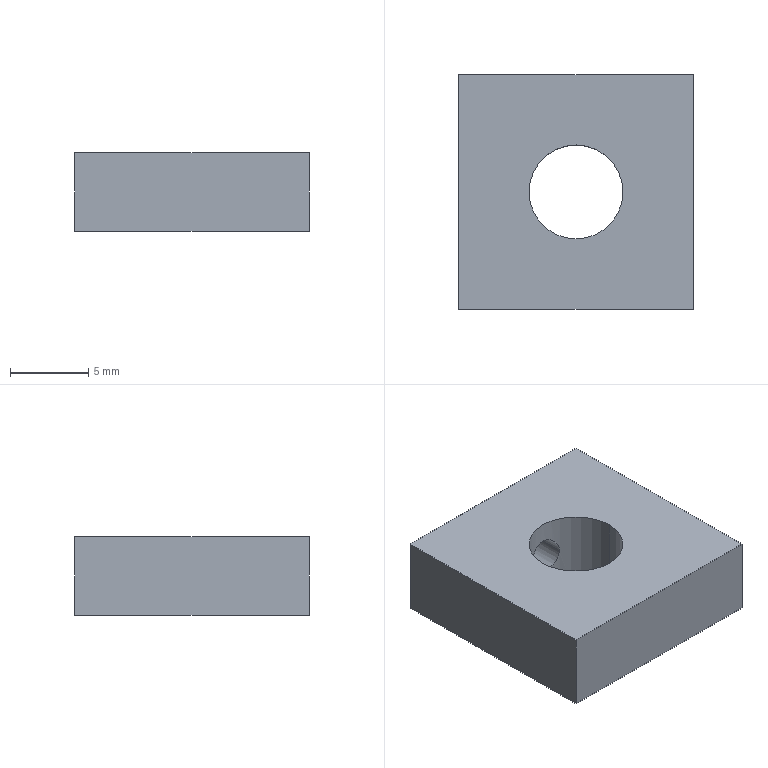Part | SolidWorks | features BaseBody 1 | 1 solid | 10 faces | box 15 x 15 x 5 mm | volume 961.952 mm3 | plane 6 | cylinder 4 | commonest cylinder face diameters 2.459 x2 6 x2
STEP:
#1=CARTESIAN_POINT('',(-105.792,-7.5,0.));
#2=VERTEX_POINT('',#1);
#3=CARTESIAN_POINT('',(-99.792,-7.5,0.));
#4=VERTEX_POINT('',#3);
#5=CARTESIAN_POINT('',(-102.792,-7.5,0.));
#6=DIRECTION('',(0.,0.,1.));
#7=DIRECTION('',(1.,0.,0.));
#8=AXIS2_PLACEMENT_3D('',#5,#6,#7);
#9=CIRCLE('',#8,3.);
#10=EDGE_CURVE('',#2,#4,#9,.T.);
#11=ORIENTED_EDGE('',*,*,#10,.F.);
#12=CARTESIAN_POINT('',(-105.792,-7.5,5.));
#13=VERTEX_POINT('',#12);
#14=CARTESIAN_POINT('',(-105.792,-7.5,-16.794));
#15=DIRECTION('',(0.,0.,1.));
#16=VECTOR('',#15,1000.);
#17=LINE('',#14,#16);
#18=EDGE_CURVE('',#2,#13,#17,.T.);
#19=ORIENTED_EDGE('',*,*,#18,.T.);
#20=CARTESIAN_POINT('',(-99.792,-7.5,5.));
#21=VERTEX_POINT('',#20);
#22=CARTESIAN_POINT('',(-102.792,-7.5,5.));
#23=DIRECTION('',(0.,0.,-1.));
#24=DIRECTION('',(1.,0.,0.));
#25=AXIS2_PLACEMENT_3D('',#22,#23,#24);
#26=CIRCLE('',#25,3.);
#27=EDGE_CURVE('',#21,#13,#26,.T.);
#28=ORIENTED_EDGE('',*,*,#27,.F.);
#29=CARTESIAN_POINT('',(-99.792,-7.5,-16.794));
#30=DIRECTION('',(0.,0.,1.));
#31=VECTOR('',#30,1000.);
#32=LINE('',#29,#31);
#33=EDGE_CURVE('',#4,#21,#32,.T.);
#34=ORIENTED_EDGE('',*,*,#33,.F.);
#35=EDGE_LOOP('',(#11,#19,#28,#34));
#36=FACE_OUTER_BOUND('',#35,.T.);
#37=CARTESIAN_POINT('',(-102.792,-7.5,-16.794));
#38=DIRECTION('',(0.,0.,1.));
#39=DIRECTION('',(1.,0.,0.));
#40=AXIS2_PLACEMENT_3D('',#37,#38,#39);
#41=CYLINDRICAL_SURFACE('',#40,3.);
#42=ADVANCED_FACE('',(#36),#41,.F.);
#43=CARTESIAN_POINT('',(-104.021,-4.764,2.5));
#44=VERTEX_POINT('',#43);
#45=CARTESIAN_POINT('',(-101.562,-4.764,2.5));
#46=VERTEX_POINT('',#45);
#47=CARTESIAN_POINT('',(-104.021,-4.764,2.5));
#48=CARTESIAN_POINT('',(-104.021,-4.764,2.336));
#49=CARTESIAN_POINT('',(-103.988,-4.748,2.174));
#50=CARTESIAN_POINT('',(-103.864,-4.697,1.878));
#51=CARTESIAN_POINT('',(-103.773,-4.663,1.743));
#52=CARTESIAN_POINT('',(-103.549,-4.595,1.518));
#53=CARTESIAN_POINT('',(-103.413,-4.561,1.427));
#54=CARTESIAN_POINT('',(-103.118,-4.514,1.304));
#55=CARTESIAN_POINT('',(-102.955,-4.5,1.271));
#56=CARTESIAN_POINT('',(-102.711,-4.5,1.27));
#57=CARTESIAN_POINT('',(-102.629,-4.503,1.279));
#58=CARTESIAN_POINT('',(-102.47,-4.516,1.311));
#59=CARTESIAN_POINT('',(-102.393,-4.526,1.334));
#60=CARTESIAN_POINT('',(-102.168,-4.562,1.428));
#61=CARTESIAN_POINT('',(-102.034,-4.595,1.519));
#62=CARTESIAN_POINT('',(-101.809,-4.663,1.744));
#63=CARTESIAN_POINT('',(-101.718,-4.698,1.879));
#64=CARTESIAN_POINT('',(-101.595,-4.748,2.175));
#65=CARTESIAN_POINT('',(-101.562,-4.764,2.338));
#66=CARTESIAN_POINT('',(-101.562,-4.764,2.5));
#67=B_SPLINE_CURVE_WITH_KNOTS('',3,(#47,#48,#49,#50,#51,#52,#53,#54,#55,#56,#57,#58,#59,#60,#61,#62,#63,#64,#65,#66),.UNSPECIFIED.,.F.,.F.,(4,2,2,2,2,2,2,2,2,4),(0.,0.0004859,0.0009718,0.001458,0.001944,0.002186,0.002429,0.002915,0.003401,0.003887),.UNSPECIFIED.);
#68=EDGE_CURVE('',#44,#46,#67,.T.);
#69=ORIENTED_EDGE('',*,*,#68,.T.);
#70=CARTESIAN_POINT('',(-101.562,0.,2.5));
#71=VERTEX_POINT('',#70);
#72=CARTESIAN_POINT('',(-101.562,-4.,2.5));
#73=DIRECTION('',(0.,1.,0.));
#74=VECTOR('',#73,1000.);
#75=LINE('',#72,#74);
#76=EDGE_CURVE('',#46,#71,#75,.T.);
#77=ORIENTED_EDGE('',*,*,#76,.T.);
#78=CARTESIAN_POINT('',(-104.021,0.,2.5));
#79=VERTEX_POINT('',#78);
#80=CARTESIAN_POINT('',(-102.792,0.,2.5));
#81=DIRECTION('',(0.,-1.,0.));
#82=DIRECTION('',(-1.,0.,0.));
#83=AXIS2_PLACEMENT_3D('',#80,#81,#82);
#84=CIRCLE('',#83,1.229);
#85=EDGE_CURVE('',#79,#71,#84,.T.);
#86=ORIENTED_EDGE('',*,*,#85,.F.);
#87=CARTESIAN_POINT('',(-104.021,-4.,2.5));
#88=DIRECTION('',(0.,1.,0.));
#89=VECTOR('',#88,1000.);
#90=LINE('',#87,#89);
#91=EDGE_CURVE('',#44,#79,#90,.T.);
#92=ORIENTED_EDGE('',*,*,#91,.F.);
#93=EDGE_LOOP('',(#69,#77,#86,#92));
#94=FACE_OUTER_BOUND('',#93,.T.);
#95=CARTESIAN_POINT('',(-102.792,-4.,2.5));
#96=DIRECTION('',(0.,1.,0.));
#97=DIRECTION('',(-1.,0.,0.));
#98=AXIS2_PLACEMENT_3D('',#95,#96,#97);
#99=CYLINDRICAL_SURFACE('',#98,1.229);
#100=ADVANCED_FACE('',(#94),#99,.F.);
#101=ORIENTED_EDGE('',*,*,#27,.T.);
#102=CARTESIAN_POINT('',(-102.792,-7.5,5.));
#103=DIRECTION('',(0.,0.,-1.));
#104=DIRECTION('',(1.,0.,0.));
#105=AXIS2_PLACEMENT_3D('',#102,#103,#104);
#106=CIRCLE('',#105,3.);
#107=EDGE_CURVE('',#13,#21,#106,.T.);
#108=ORIENTED_EDGE('',*,*,#107,.T.);
#109=EDGE_LOOP('',(#101,#108));
#110=FACE_BOUND('',#109,.T.);
#111=CARTESIAN_POINT('',(-95.292,-15.,5.));
#112=VERTEX_POINT('',#111);
#113=CARTESIAN_POINT('',(-95.292,0.,5.));
#114=VERTEX_POINT('',#113);
#115=CARTESIAN_POINT('',(-95.292,-7.5,5.));
#116=DIRECTION('',(0.,1.,0.));
#117=VECTOR('',#116,1000.);
#118=LINE('',#115,#117);
#119=EDGE_CURVE('',#112,#114,#118,.T.);
#120=ORIENTED_EDGE('',*,*,#119,.T.);
#121=CARTESIAN_POINT('',(-110.292,0.,5.));
#122=VERTEX_POINT('',#121);
#123=CARTESIAN_POINT('',(-102.792,0.,5.));
#124=DIRECTION('',(-1.,0.,0.));
#125=VECTOR('',#124,1000.);
#126=LINE('',#123,#125);
#127=EDGE_CURVE('',#114,#122,#126,.T.);
#128=ORIENTED_EDGE('',*,*,#127,.T.);
#129=CARTESIAN_POINT('',(-110.292,-15.,5.));
#130=VERTEX_POINT('',#129);
#131=CARTESIAN_POINT('',(-110.292,-7.5,5.));
#132=DIRECTION('',(0.,-1.,0.));
#133=VECTOR('',#132,1000.);
#134=LINE('',#131,#133);
#135=EDGE_CURVE('',#122,#130,#134,.T.);
#136=ORIENTED_EDGE('',*,*,#135,.T.);
#137=CARTESIAN_POINT('',(-102.792,-15.,5.));
#138=DIRECTION('',(1.,0.,0.));
#139=VECTOR('',#138,1000.);
#140=LINE('',#137,#139);
#141=EDGE_CURVE('',#130,#112,#140,.T.);
#142=ORIENTED_EDGE('',*,*,#141,.T.);
#143=EDGE_LOOP('',(#120,#128,#136,#142));
#144=FACE_OUTER_BOUND('',#143,.T.);
#145=CARTESIAN_POINT('',(-102.792,-7.5,5.));
#146=DIRECTION('',(0.,0.,1.));
#147=DIRECTION('',(1.,0.,0.));
#148=AXIS2_PLACEMENT_3D('',#145,#146,#147);
#149=PLANE('',#148);
#150=ADVANCED_FACE('',(#110,#144),#149,.T.);
#151=ORIENTED_EDGE('',*,*,#18,.F.);
#152=CARTESIAN_POINT('',(-102.792,-7.5,0.));
#153=DIRECTION('',(0.,0.,1.));
#154=DIRECTION('',(1.,0.,0.));
#155=AXIS2_PLACEMENT_3D('',#152,#153,#154);
#156=CIRCLE('',#155,3.);
#157=EDGE_CURVE('',#4,#2,#156,.T.);
#158=ORIENTED_EDGE('',*,*,#157,.F.);
#159=ORIENTED_EDGE('',*,*,#33,.T.);
#160=ORIENTED_EDGE('',*,*,#107,.F.);
#161=EDGE_LOOP('',(#151,#158,#159,#160));
#162=FACE_OUTER_BOUND('',#161,.T.);
#163=ORIENTED_EDGE('',*,*,#68,.F.);
#164=CARTESIAN_POINT('',(-101.562,-4.764,2.5));
#165=CARTESIAN_POINT('',(-101.562,-4.764,2.662));
#166=CARTESIAN_POINT('',(-101.595,-4.748,2.825));
#167=CARTESIAN_POINT('',(-101.719,-4.698,3.122));
#168=CARTESIAN_POINT('',(-101.809,-4.663,3.256));
#169=CARTESIAN_POINT('',(-101.979,-4.612,3.426));
#170=CARTESIAN_POINT('',(-102.041,-4.595,3.477));
#171=CARTESIAN_POINT('',(-102.173,-4.564,3.565));
#172=CARTESIAN_POINT('',(-102.244,-4.549,3.604));
#173=CARTESIAN_POINT('',(-102.393,-4.526,3.666));
#174=CARTESIAN_POINT('',(-102.47,-4.516,3.689));
#175=CARTESIAN_POINT('',(-102.628,-4.503,3.721));
#176=CARTESIAN_POINT('',(-102.711,-4.5,3.729));
#177=CARTESIAN_POINT('',(-102.954,-4.5,3.73));
#178=CARTESIAN_POINT('',(-103.117,-4.514,3.697));
#179=CARTESIAN_POINT('',(-103.414,-4.561,3.573));
#180=CARTESIAN_POINT('',(-103.549,-4.595,3.482));
#181=CARTESIAN_POINT('',(-103.774,-4.663,3.256));
#182=CARTESIAN_POINT('',(-103.864,-4.697,3.123));
#183=CARTESIAN_POINT('',(-103.989,-4.748,2.824));
#184=CARTESIAN_POINT('',(-104.021,-4.764,2.664));
#185=CARTESIAN_POINT('',(-104.021,-4.764,2.5));
#186=B_SPLINE_CURVE_WITH_KNOTS('',3,(#164,#165,#166,#167,#168,#169,#170,#171,#172,#173,#174,#175,#176,#177,#178,#179,#180,#181,#182,#183,#184,#185),.UNSPECIFIED.,.F.,.F.,(4,2,2,2,2,2,2,2,2,2,4),(0.003887,0.004373,0.004858,0.005101,0.005344,0.005586,0.005829,0.006315,0.0068,0.007286,0.007771),.UNSPECIFIED.);
#187=EDGE_CURVE('',#46,#44,#186,.T.);
#188=ORIENTED_EDGE('',*,*,#187,.F.);
#189=EDGE_LOOP('',(#163,#188));
#190=FACE_BOUND('',#189,.T.);
#191=CARTESIAN_POINT('',(-102.792,-7.5,-16.794));
#192=DIRECTION('',(0.,0.,1.));
#193=DIRECTION('',(1.,0.,0.));
#194=AXIS2_PLACEMENT_3D('',#191,#192,#193);
#195=CYLINDRICAL_SURFACE('',#194,3.);
#196=ADVANCED_FACE('',(#162,#190),#195,.F.);
#197=ORIENTED_EDGE('',*,*,#85,.T.);
#198=CARTESIAN_POINT('',(-102.792,0.,2.5));
#199=DIRECTION('',(0.,-1.,0.));
#200=DIRECTION('',(-1.,0.,0.));
#201=AXIS2_PLACEMENT_3D('',#198,#199,#200);
#202=CIRCLE('',#201,1.229);
#203=EDGE_CURVE('',#71,#79,#202,.T.);
#204=ORIENTED_EDGE('',*,*,#203,.T.);
#205=EDGE_LOOP('',(#197,#204));
#206=FACE_BOUND('',#205,.T.);
#207=CARTESIAN_POINT('',(-95.292,0.,0.));
#208=VERTEX_POINT('',#207);
#209=CARTESIAN_POINT('',(-110.292,0.,0.));
#210=VERTEX_POINT('',#209);
#211=CARTESIAN_POINT('',(-110.292,0.,0.));
#212=DIRECTION('',(-1.,0.,0.));
#213=VECTOR('',#212,1000.);
#214=LINE('',#211,#213);
#215=EDGE_CURVE('',#208,#210,#214,.T.);
#216=ORIENTED_EDGE('',*,*,#215,.T.);
#217=CARTESIAN_POINT('',(-110.292,0.,0.));
#218=DIRECTION('',(0.,0.,1.));
#219=VECTOR('',#218,1000.);
#220=LINE('',#217,#219);
#221=EDGE_CURVE('',#210,#122,#220,.T.);
#222=ORIENTED_EDGE('',*,*,#221,.T.);
#223=ORIENTED_EDGE('',*,*,#127,.F.);
#224=CARTESIAN_POINT('',(-95.292,0.,0.));
#225=DIRECTION('',(0.,0.,-1.));
#226=VECTOR('',#225,1000.);
#227=LINE('',#224,#226);
#228=EDGE_CURVE('',#114,#208,#227,.T.);
#229=ORIENTED_EDGE('',*,*,#228,.T.);
#230=EDGE_LOOP('',(#216,#222,#223,#229));
#231=FACE_OUTER_BOUND('',#230,.T.);
#232=CARTESIAN_POINT('',(-110.292,0.,0.));
#233=DIRECTION('',(0.,1.,0.));
#234=DIRECTION('',(0.,0.,1.));
#235=AXIS2_PLACEMENT_3D('',#232,#233,#234);
#236=PLANE('',#235);
#237=ADVANCED_FACE('',(#206,#231),#236,.T.);
#238=CARTESIAN_POINT('',(-95.292,-15.,0.));
#239=VERTEX_POINT('',#238);
#240=CARTESIAN_POINT('',(-95.292,0.,0.));
#241=DIRECTION('',(0.,1.,0.));
#242=VECTOR('',#241,1000.);
#243=LINE('',#240,#242);
#244=EDGE_CURVE('',#239,#208,#243,.T.);
#245=ORIENTED_EDGE('',*,*,#244,.T.);
#246=ORIENTED_EDGE('',*,*,#228,.F.);
#247=ORIENTED_EDGE('',*,*,#119,.F.);
#248=CARTESIAN_POINT('',(-95.292,-15.,0.));
#249=DIRECTION('',(0.,0.,-1.));
#250=VECTOR('',#249,1000.);
#251=LINE('',#248,#250);
#252=EDGE_CURVE('',#112,#239,#251,.T.);
#253=ORIENTED_EDGE('',*,*,#252,.T.);
#254=EDGE_LOOP('',(#245,#246,#247,#253));
#255=FACE_OUTER_BOUND('',#254,.T.);
#256=CARTESIAN_POINT('',(-95.292,0.,0.));
#257=DIRECTION('',(1.,0.,0.));
#258=DIRECTION('',(0.,0.,-1.));
#259=AXIS2_PLACEMENT_3D('',#256,#257,#258);
#260=PLANE('',#259);
#261=ADVANCED_FACE('',(#255),#260,.T.);
#262=CARTESIAN_POINT('',(-110.292,-15.,0.));
#263=VERTEX_POINT('',#262);
#264=CARTESIAN_POINT('',(-95.292,-15.,0.));
#265=DIRECTION('',(1.,0.,0.));
#266=VECTOR('',#265,1000.);
#267=LINE('',#264,#266);
#268=EDGE_CURVE('',#263,#239,#267,.T.);
#269=ORIENTED_EDGE('',*,*,#268,.T.);
#270=ORIENTED_EDGE('',*,*,#252,.F.);
#271=ORIENTED_EDGE('',*,*,#141,.F.);
#272=CARTESIAN_POINT('',(-110.292,-15.,0.));
#273=DIRECTION('',(0.,0.,-1.));
#274=VECTOR('',#273,1000.);
#275=LINE('',#272,#274);
#276=EDGE_CURVE('',#130,#263,#275,.T.);
#277=ORIENTED_EDGE('',*,*,#276,.T.);
#278=EDGE_LOOP('',(#269,#270,#271,#277));
#279=FACE_OUTER_BOUND('',#278,.T.);
#280=CARTESIAN_POINT('',(-95.292,-15.,0.));
#281=DIRECTION('',(0.,-1.,0.));
#282=DIRECTION('',(0.,0.,-1.));
#283=AXIS2_PLACEMENT_3D('',#280,#281,#282);
#284=PLANE('',#283);
#285=ADVANCED_FACE('',(#279),#284,.T.);
#286=CARTESIAN_POINT('',(-110.292,-15.,0.));
#287=DIRECTION('',(0.,-1.,0.));
#288=VECTOR('',#287,1000.);
#289=LINE('',#286,#288);
#290=EDGE_CURVE('',#210,#263,#289,.T.);
#291=ORIENTED_EDGE('',*,*,#290,.T.);
#292=ORIENTED_EDGE('',*,*,#276,.F.);
#293=ORIENTED_EDGE('',*,*,#135,.F.);
#294=ORIENTED_EDGE('',*,*,#221,.F.);
#295=EDGE_LOOP('',(#291,#292,#293,#294));
#296=FACE_OUTER_BOUND('',#295,.T.);
#297=CARTESIAN_POINT('',(-110.292,-15.,0.));
#298=DIRECTION('',(-1.,0.,0.));
#299=DIRECTION('',(0.,0.,1.));
#300=AXIS2_PLACEMENT_3D('',#297,#298,#299);
#301=PLANE('',#300);
#302=ADVANCED_FACE('',(#296),#301,.T.);
#303=ORIENTED_EDGE('',*,*,#76,.F.);
#304=ORIENTED_EDGE('',*,*,#187,.T.);
#305=ORIENTED_EDGE('',*,*,#91,.T.);
#306=ORIENTED_EDGE('',*,*,#203,.F.);
#307=EDGE_LOOP('',(#303,#304,#305,#306));
#308=FACE_OUTER_BOUND('',#307,.T.);
#309=CARTESIAN_POINT('',(-102.792,-4.,2.5));
#310=DIRECTION('',(0.,1.,0.));
#311=DIRECTION('',(-1.,0.,0.));
#312=AXIS2_PLACEMENT_3D('',#309,#310,#311);
#313=CYLINDRICAL_SURFACE('',#312,1.229);
#314=ADVANCED_FACE('',(#308),#313,.F.);
#315=ORIENTED_EDGE('',*,*,#157,.T.);
#316=ORIENTED_EDGE('',*,*,#10,.T.);
#317=EDGE_LOOP('',(#315,#316));
#318=FACE_BOUND('',#317,.T.);
#319=ORIENTED_EDGE('',*,*,#290,.F.);
#320=ORIENTED_EDGE('',*,*,#215,.F.);
#321=ORIENTED_EDGE('',*,*,#244,.F.);
#322=ORIENTED_EDGE('',*,*,#268,.F.);
#323=EDGE_LOOP('',(#319,#320,#321,#322));
#324=FACE_OUTER_BOUND('',#323,.T.);
#325=CARTESIAN_POINT('',(-102.792,-7.5,0.));
#326=DIRECTION('',(0.,0.,1.));
#327=DIRECTION('',(1.,0.,0.));
#328=AXIS2_PLACEMENT_3D('',#325,#326,#327);
#329=PLANE('',#328);
#330=ADVANCED_FACE('',(#318,#324),#329,.F.);
#331=CLOSED_SHELL('',(#42,#100,#150,#196,#237,#261,#285,#302,#314,#330));
#332=MANIFOLD_SOLID_BREP('',#331);
#333=CARTESIAN_POINT('',(0.,0.,0.));
#334=DIRECTION('',(0.,0.,1.));
#335=DIRECTION('',(1.,0.,0.));
#336=AXIS2_PLACEMENT_3D('',#333,#334,#335);
#337=(LENGTH_UNIT()NAMED_UNIT(*)SI_UNIT(.MILLI.,.METRE.));
#338=UNCERTAINTY_MEASURE_WITH_UNIT(LENGTH_MEASURE(0.00001),#337,'','');
#339=(NAMED_UNIT(*)PLANE_ANGLE_UNIT()SI_UNIT($,.RADIAN.));
#340=(NAMED_UNIT(*)SI_UNIT($,.STERADIAN.)SOLID_ANGLE_UNIT());
#341=(GEOMETRIC_REPRESENTATION_CONTEXT(3)GLOBAL_UNCERTAINTY_ASSIGNED_CONTEXT((#338))GLOBAL_UNIT_ASSIGNED_CONTEXT((#337,#339,#340))REPRESENTATION_CONTEXT('',''));
#342=ADVANCED_BREP_SHAPE_REPRESENTATION('',(#332,#336),#341);